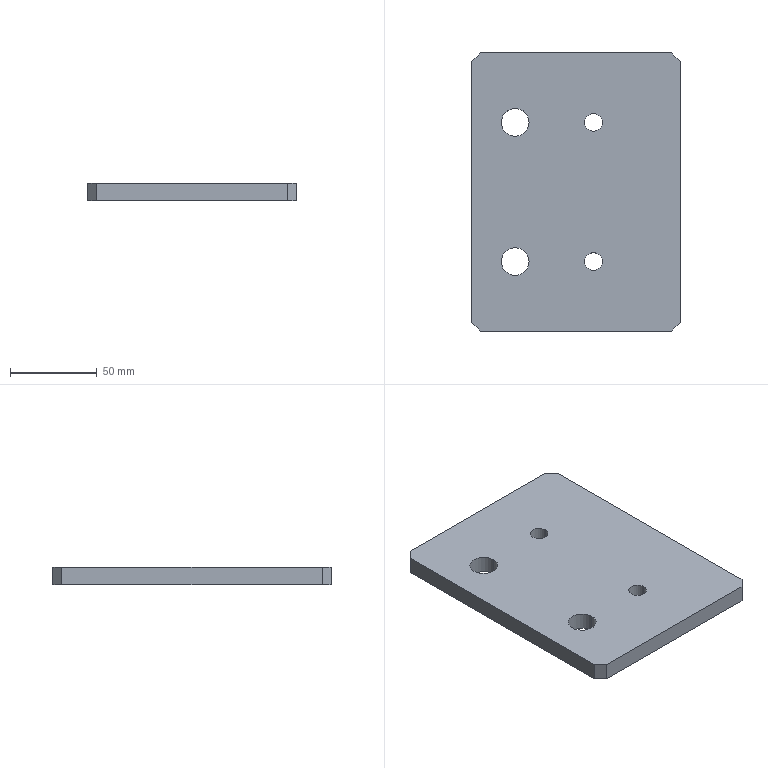Part | STEP file | 中转釜楼梯底Plate 1 | 1 solid | 18 faces | box 120 x 160 x 10 mm | volume 185845 mm3 | plane 10 | cylinder 8 | commonest cylinder face diameters 10.2 x4 16 x4
STEP:
#1=CARTESIAN_POINT('',(0.,0.,0.));
#2=DIRECTION('',(0.,0.,1.));
#3=DIRECTION('',(1.,0.,0.));
#4=AXIS2_PLACEMENT_3D('',#1,#2,#3);
#5=CARTESIAN_POINT('',(15.1,120.,0.));
#6=VERTEX_POINT('',#5);
#7=CARTESIAN_POINT('',(15.1,120.,10.));
#8=VERTEX_POINT('',#7);
#9=CARTESIAN_POINT('',(15.1,120.,10.));
#10=DIRECTION('',(0.,0.,1.));
#11=VECTOR('',#10,1.);
#12=LINE('',#9,#11);
#13=CARTESIAN_POINT('',(10.,120.,10.));
#14=DIRECTION('',(0.,0.,1.));
#15=DIRECTION('',(1.,0.,0.));
#16=AXIS2_PLACEMENT_3D('',#13,#14,#15);
#17=CYLINDRICAL_SURFACE('',#16,5.1);
#18=CARTESIAN_POINT('',(6.283,0.));
#19=DIRECTION('',(0.,1.));
#20=VECTOR('',#19,1.);
#21=LINE('',#18,#20);
#22=(GEOMETRIC_REPRESENTATION_CONTEXT(2)PARAMETRIC_REPRESENTATION_CONTEXT()REPRESENTATION_CONTEXT('',''));
#23=DEFINITIONAL_REPRESENTATION('',(#21),#22);
#24=PCURVE('',#17,#23);
#25=CARTESIAN_POINT('',(10.,120.,10.));
#26=DIRECTION('',(0.,0.,1.));
#27=DIRECTION('',(1.,0.,0.));
#28=AXIS2_PLACEMENT_3D('',#25,#26,#27);
#29=CYLINDRICAL_SURFACE('',#28,5.1);
#30=CARTESIAN_POINT('',(0.,0.));
#31=DIRECTION('',(0.,1.));
#32=VECTOR('',#31,1.);
#33=LINE('',#30,#32);
#34=(GEOMETRIC_REPRESENTATION_CONTEXT(2)PARAMETRIC_REPRESENTATION_CONTEXT()REPRESENTATION_CONTEXT('',''));
#35=DEFINITIONAL_REPRESENTATION('',(#33),#34);
#36=PCURVE('',#29,#35);
#37=SURFACE_CURVE('',#12,(#24,#36),.PCURVE_S1.);
#38=EDGE_CURVE('',#6,#8,#37,.T.);
#39=ORIENTED_EDGE('',*,*,#38,.T.);
#40=CARTESIAN_POINT('',(4.9,120.,10.));
#41=VERTEX_POINT('',#40);
#42=CARTESIAN_POINT('',(10.,120.,10.));
#43=DIRECTION('',(0.,0.,1.));
#44=DIRECTION('',(1.,0.,0.));
#45=AXIS2_PLACEMENT_3D('',#42,#43,#44);
#46=CIRCLE('',#45,5.1);
#47=CARTESIAN_POINT('',(0.,0.));
#48=DIRECTION('',(1.,0.));
#49=VECTOR('',#48,1.);
#50=LINE('',#47,#49);
#51=(GEOMETRIC_REPRESENTATION_CONTEXT(2)PARAMETRIC_REPRESENTATION_CONTEXT()REPRESENTATION_CONTEXT('',''));
#52=DEFINITIONAL_REPRESENTATION('',(#50),#51);
#53=PCURVE('',#17,#52);
#54=CARTESIAN_POINT('',(0.,0.,10.));
#55=DIRECTION('',(0.,0.,1.));
#56=DIRECTION('',(1.,0.,0.));
#57=AXIS2_PLACEMENT_3D('',#54,#55,#56);
#58=PLANE('',#57);
#59=CARTESIAN_POINT('',(10.,120.));
#60=DIRECTION('',(1.,0.));
#61=AXIS2_PLACEMENT_2D('',#59,#60);
#62=CIRCLE('',#61,5.1);
#63=(GEOMETRIC_REPRESENTATION_CONTEXT(2)PARAMETRIC_REPRESENTATION_CONTEXT()REPRESENTATION_CONTEXT('',''));
#64=DEFINITIONAL_REPRESENTATION('',(#62),#63);
#65=PCURVE('',#58,#64);
#66=SURFACE_CURVE('',#46,(#53,#65),.PCURVE_S1.);
#67=EDGE_CURVE('',#41,#8,#66,.T.);
#68=ORIENTED_EDGE('',*,*,#67,.F.);
#69=CARTESIAN_POINT('',(4.9,120.,0.));
#70=VERTEX_POINT('',#69);
#71=CARTESIAN_POINT('',(4.9,120.,10.));
#72=DIRECTION('',(0.,0.,1.));
#73=VECTOR('',#72,1.);
#74=LINE('',#71,#73);
#75=CARTESIAN_POINT('',(3.142,0.));
#76=DIRECTION('',(0.,1.));
#77=VECTOR('',#76,1.);
#78=LINE('',#75,#77);
#79=(GEOMETRIC_REPRESENTATION_CONTEXT(2)PARAMETRIC_REPRESENTATION_CONTEXT()REPRESENTATION_CONTEXT('',''));
#80=DEFINITIONAL_REPRESENTATION('',(#78),#79);
#81=PCURVE('',#17,#80);
#82=CARTESIAN_POINT('',(3.142,0.));
#83=DIRECTION('',(0.,1.));
#84=VECTOR('',#83,1.);
#85=LINE('',#82,#84);
#86=(GEOMETRIC_REPRESENTATION_CONTEXT(2)PARAMETRIC_REPRESENTATION_CONTEXT()REPRESENTATION_CONTEXT('',''));
#87=DEFINITIONAL_REPRESENTATION('',(#85),#86);
#88=PCURVE('',#29,#87);
#89=SURFACE_CURVE('',#74,(#81,#88),.PCURVE_S1.);
#90=EDGE_CURVE('',#70,#41,#89,.T.);
#91=ORIENTED_EDGE('',*,*,#90,.F.);
#92=CARTESIAN_POINT('',(10.,120.,0.));
#93=DIRECTION('',(0.,0.,1.));
#94=DIRECTION('',(1.,0.,0.));
#95=AXIS2_PLACEMENT_3D('',#92,#93,#94);
#96=CIRCLE('',#95,5.1);
#97=CARTESIAN_POINT('',(0.,-10.));
#98=DIRECTION('',(1.,0.));
#99=VECTOR('',#98,1.);
#100=LINE('',#97,#99);
#101=(GEOMETRIC_REPRESENTATION_CONTEXT(2)PARAMETRIC_REPRESENTATION_CONTEXT()REPRESENTATION_CONTEXT('',''));
#102=DEFINITIONAL_REPRESENTATION('',(#100),#101);
#103=PCURVE('',#17,#102);
#104=CARTESIAN_POINT('',(0.,0.,0.));
#105=DIRECTION('',(0.,0.,1.));
#106=DIRECTION('',(1.,0.,0.));
#107=AXIS2_PLACEMENT_3D('',#104,#105,#106);
#108=PLANE('',#107);
#109=CARTESIAN_POINT('',(10.,120.));
#110=DIRECTION('',(1.,0.));
#111=AXIS2_PLACEMENT_2D('',#109,#110);
#112=CIRCLE('',#111,5.1);
#113=(GEOMETRIC_REPRESENTATION_CONTEXT(2)PARAMETRIC_REPRESENTATION_CONTEXT()REPRESENTATION_CONTEXT('',''));
#114=DEFINITIONAL_REPRESENTATION('',(#112),#113);
#115=PCURVE('',#108,#114);
#116=SURFACE_CURVE('',#96,(#103,#115),.PCURVE_S1.);
#117=EDGE_CURVE('',#70,#6,#116,.T.);
#118=ORIENTED_EDGE('',*,*,#117,.T.);
#119=EDGE_LOOP('',(#39,#68,#91,#118));
#120=FACE_BOUND('',#119,.F.);
#121=ADVANCED_FACE('',(#120),#17,.F.);
#122=CARTESIAN_POINT('',(15.1,40.,0.));
#123=VERTEX_POINT('',#122);
#124=CARTESIAN_POINT('',(15.1,40.,10.));
#125=VERTEX_POINT('',#124);
#126=CARTESIAN_POINT('',(15.1,40.,10.));
#127=DIRECTION('',(0.,0.,1.));
#128=VECTOR('',#127,1.);
#129=LINE('',#126,#128);
#130=CARTESIAN_POINT('',(10.,40.,10.));
#131=DIRECTION('',(0.,0.,1.));
#132=DIRECTION('',(1.,0.,0.));
#133=AXIS2_PLACEMENT_3D('',#130,#131,#132);
#134=CYLINDRICAL_SURFACE('',#133,5.1);
#135=CARTESIAN_POINT('',(6.283,0.));
#136=DIRECTION('',(0.,1.));
#137=VECTOR('',#136,1.);
#138=LINE('',#135,#137);
#139=(GEOMETRIC_REPRESENTATION_CONTEXT(2)PARAMETRIC_REPRESENTATION_CONTEXT()REPRESENTATION_CONTEXT('',''));
#140=DEFINITIONAL_REPRESENTATION('',(#138),#139);
#141=PCURVE('',#134,#140);
#142=CARTESIAN_POINT('',(10.,40.,10.));
#143=DIRECTION('',(0.,0.,1.));
#144=DIRECTION('',(1.,0.,0.));
#145=AXIS2_PLACEMENT_3D('',#142,#143,#144);
#146=CYLINDRICAL_SURFACE('',#145,5.1);
#147=CARTESIAN_POINT('',(0.,0.));
#148=DIRECTION('',(0.,1.));
#149=VECTOR('',#148,1.);
#150=LINE('',#147,#149);
#151=(GEOMETRIC_REPRESENTATION_CONTEXT(2)PARAMETRIC_REPRESENTATION_CONTEXT()REPRESENTATION_CONTEXT('',''));
#152=DEFINITIONAL_REPRESENTATION('',(#150),#151);
#153=PCURVE('',#146,#152);
#154=SURFACE_CURVE('',#129,(#141,#153),.PCURVE_S1.);
#155=EDGE_CURVE('',#123,#125,#154,.T.);
#156=ORIENTED_EDGE('',*,*,#155,.T.);
#157=CARTESIAN_POINT('',(4.9,40.,10.));
#158=VERTEX_POINT('',#157);
#159=CARTESIAN_POINT('',(10.,40.,10.));
#160=DIRECTION('',(0.,0.,1.));
#161=DIRECTION('',(1.,0.,0.));
#162=AXIS2_PLACEMENT_3D('',#159,#160,#161);
#163=CIRCLE('',#162,5.1);
#164=CARTESIAN_POINT('',(0.,0.));
#165=DIRECTION('',(1.,0.));
#166=VECTOR('',#165,1.);
#167=LINE('',#164,#166);
#168=(GEOMETRIC_REPRESENTATION_CONTEXT(2)PARAMETRIC_REPRESENTATION_CONTEXT()REPRESENTATION_CONTEXT('',''));
#169=DEFINITIONAL_REPRESENTATION('',(#167),#168);
#170=PCURVE('',#134,#169);
#171=CARTESIAN_POINT('',(10.,40.));
#172=DIRECTION('',(1.,0.));
#173=AXIS2_PLACEMENT_2D('',#171,#172);
#174=CIRCLE('',#173,5.1);
#175=(GEOMETRIC_REPRESENTATION_CONTEXT(2)PARAMETRIC_REPRESENTATION_CONTEXT()REPRESENTATION_CONTEXT('',''));
#176=DEFINITIONAL_REPRESENTATION('',(#174),#175);
#177=PCURVE('',#58,#176);
#178=SURFACE_CURVE('',#163,(#170,#177),.PCURVE_S1.);
#179=EDGE_CURVE('',#158,#125,#178,.T.);
#180=ORIENTED_EDGE('',*,*,#179,.F.);
#181=CARTESIAN_POINT('',(4.9,40.,0.));
#182=VERTEX_POINT('',#181);
#183=CARTESIAN_POINT('',(4.9,40.,10.));
#184=DIRECTION('',(0.,0.,1.));
#185=VECTOR('',#184,1.);
#186=LINE('',#183,#185);
#187=CARTESIAN_POINT('',(3.142,0.));
#188=DIRECTION('',(0.,1.));
#189=VECTOR('',#188,1.);
#190=LINE('',#187,#189);
#191=(GEOMETRIC_REPRESENTATION_CONTEXT(2)PARAMETRIC_REPRESENTATION_CONTEXT()REPRESENTATION_CONTEXT('',''));
#192=DEFINITIONAL_REPRESENTATION('',(#190),#191);
#193=PCURVE('',#134,#192);
#194=CARTESIAN_POINT('',(3.142,0.));
#195=DIRECTION('',(0.,1.));
#196=VECTOR('',#195,1.);
#197=LINE('',#194,#196);
#198=(GEOMETRIC_REPRESENTATION_CONTEXT(2)PARAMETRIC_REPRESENTATION_CONTEXT()REPRESENTATION_CONTEXT('',''));
#199=DEFINITIONAL_REPRESENTATION('',(#197),#198);
#200=PCURVE('',#146,#199);
#201=SURFACE_CURVE('',#186,(#193,#200),.PCURVE_S1.);
#202=EDGE_CURVE('',#182,#158,#201,.T.);
#203=ORIENTED_EDGE('',*,*,#202,.F.);
#204=CARTESIAN_POINT('',(10.,40.,0.));
#205=DIRECTION('',(0.,0.,1.));
#206=DIRECTION('',(1.,0.,0.));
#207=AXIS2_PLACEMENT_3D('',#204,#205,#206);
#208=CIRCLE('',#207,5.1);
#209=CARTESIAN_POINT('',(0.,-10.));
#210=DIRECTION('',(1.,0.));
#211=VECTOR('',#210,1.);
#212=LINE('',#209,#211);
#213=(GEOMETRIC_REPRESENTATION_CONTEXT(2)PARAMETRIC_REPRESENTATION_CONTEXT()REPRESENTATION_CONTEXT('',''));
#214=DEFINITIONAL_REPRESENTATION('',(#212),#213);
#215=PCURVE('',#134,#214);
#216=CARTESIAN_POINT('',(10.,40.));
#217=DIRECTION('',(1.,0.));
#218=AXIS2_PLACEMENT_2D('',#216,#217);
#219=CIRCLE('',#218,5.1);
#220=(GEOMETRIC_REPRESENTATION_CONTEXT(2)PARAMETRIC_REPRESENTATION_CONTEXT()REPRESENTATION_CONTEXT('',''));
#221=DEFINITIONAL_REPRESENTATION('',(#219),#220);
#222=PCURVE('',#108,#221);
#223=SURFACE_CURVE('',#208,(#215,#222),.PCURVE_S1.);
#224=EDGE_CURVE('',#182,#123,#223,.T.);
#225=ORIENTED_EDGE('',*,*,#224,.T.);
#226=EDGE_LOOP('',(#156,#180,#203,#225));
#227=FACE_BOUND('',#226,.F.);
#228=ADVANCED_FACE('',(#227),#134,.F.);
#229=CARTESIAN_POINT('',(-27.,40.,0.));
#230=VERTEX_POINT('',#229);
#231=CARTESIAN_POINT('',(-27.,40.,10.));
#232=VERTEX_POINT('',#231);
#233=CARTESIAN_POINT('',(-27.,40.,10.));
#234=DIRECTION('',(0.,0.,1.));
#235=VECTOR('',#234,1.);
#236=LINE('',#233,#235);
#237=CARTESIAN_POINT('',(-35.,40.,10.));
#238=DIRECTION('',(0.,0.,1.));
#239=DIRECTION('',(1.,0.,0.));
#240=AXIS2_PLACEMENT_3D('',#237,#238,#239);
#241=CYLINDRICAL_SURFACE('',#240,8.);
#242=CARTESIAN_POINT('',(6.283,0.));
#243=DIRECTION('',(0.,1.));
#244=VECTOR('',#243,1.);
#245=LINE('',#242,#244);
#246=(GEOMETRIC_REPRESENTATION_CONTEXT(2)PARAMETRIC_REPRESENTATION_CONTEXT()REPRESENTATION_CONTEXT('',''));
#247=DEFINITIONAL_REPRESENTATION('',(#245),#246);
#248=PCURVE('',#241,#247);
#249=CARTESIAN_POINT('',(-35.,40.,10.));
#250=DIRECTION('',(0.,0.,1.));
#251=DIRECTION('',(1.,0.,0.));
#252=AXIS2_PLACEMENT_3D('',#249,#250,#251);
#253=CYLINDRICAL_SURFACE('',#252,8.);
#254=CARTESIAN_POINT('',(0.,0.));
#255=DIRECTION('',(0.,1.));
#256=VECTOR('',#255,1.);
#257=LINE('',#254,#256);
#258=(GEOMETRIC_REPRESENTATION_CONTEXT(2)PARAMETRIC_REPRESENTATION_CONTEXT()REPRESENTATION_CONTEXT('',''));
#259=DEFINITIONAL_REPRESENTATION('',(#257),#258);
#260=PCURVE('',#253,#259);
#261=SURFACE_CURVE('',#236,(#248,#260),.PCURVE_S1.);
#262=EDGE_CURVE('',#230,#232,#261,.T.);
#263=ORIENTED_EDGE('',*,*,#262,.T.);
#264=CARTESIAN_POINT('',(-43.,40.,10.));
#265=VERTEX_POINT('',#264);
#266=CARTESIAN_POINT('',(-35.,40.,10.));
#267=DIRECTION('',(0.,0.,1.));
#268=DIRECTION('',(1.,0.,0.));
#269=AXIS2_PLACEMENT_3D('',#266,#267,#268);
#270=CIRCLE('',#269,8.);
#271=CARTESIAN_POINT('',(0.,0.));
#272=DIRECTION('',(1.,0.));
#273=VECTOR('',#272,1.);
#274=LINE('',#271,#273);
#275=(GEOMETRIC_REPRESENTATION_CONTEXT(2)PARAMETRIC_REPRESENTATION_CONTEXT()REPRESENTATION_CONTEXT('',''));
#276=DEFINITIONAL_REPRESENTATION('',(#274),#275);
#277=PCURVE('',#241,#276);
#278=CARTESIAN_POINT('',(-35.,40.));
#279=DIRECTION('',(1.,0.));
#280=AXIS2_PLACEMENT_2D('',#278,#279);
#281=CIRCLE('',#280,8.);
#282=(GEOMETRIC_REPRESENTATION_CONTEXT(2)PARAMETRIC_REPRESENTATION_CONTEXT()REPRESENTATION_CONTEXT('',''));
#283=DEFINITIONAL_REPRESENTATION('',(#281),#282);
#284=PCURVE('',#58,#283);
#285=SURFACE_CURVE('',#270,(#277,#284),.PCURVE_S1.);
#286=EDGE_CURVE('',#265,#232,#285,.T.);
#287=ORIENTED_EDGE('',*,*,#286,.F.);
#288=CARTESIAN_POINT('',(-43.,40.,0.));
#289=VERTEX_POINT('',#288);
#290=CARTESIAN_POINT('',(-43.,40.,10.));
#291=DIRECTION('',(0.,0.,1.));
#292=VECTOR('',#291,1.);
#293=LINE('',#290,#292);
#294=CARTESIAN_POINT('',(3.142,0.));
#295=DIRECTION('',(0.,1.));
#296=VECTOR('',#295,1.);
#297=LINE('',#294,#296);
#298=(GEOMETRIC_REPRESENTATION_CONTEXT(2)PARAMETRIC_REPRESENTATION_CONTEXT()REPRESENTATION_CONTEXT('',''));
#299=DEFINITIONAL_REPRESENTATION('',(#297),#298);
#300=PCURVE('',#241,#299);
#301=CARTESIAN_POINT('',(3.142,0.));
#302=DIRECTION('',(0.,1.));
#303=VECTOR('',#302,1.);
#304=LINE('',#301,#303);
#305=(GEOMETRIC_REPRESENTATION_CONTEXT(2)PARAMETRIC_REPRESENTATION_CONTEXT()REPRESENTATION_CONTEXT('',''));
#306=DEFINITIONAL_REPRESENTATION('',(#304),#305);
#307=PCURVE('',#253,#306);
#308=SURFACE_CURVE('',#293,(#300,#307),.PCURVE_S1.);
#309=EDGE_CURVE('',#289,#265,#308,.T.);
#310=ORIENTED_EDGE('',*,*,#309,.F.);
#311=CARTESIAN_POINT('',(-35.,40.,0.));
#312=DIRECTION('',(0.,0.,1.));
#313=DIRECTION('',(1.,0.,0.));
#314=AXIS2_PLACEMENT_3D('',#311,#312,#313);
#315=CIRCLE('',#314,8.);
#316=CARTESIAN_POINT('',(0.,-10.));
#317=DIRECTION('',(1.,0.));
#318=VECTOR('',#317,1.);
#319=LINE('',#316,#318);
#320=(GEOMETRIC_REPRESENTATION_CONTEXT(2)PARAMETRIC_REPRESENTATION_CONTEXT()REPRESENTATION_CONTEXT('',''));
#321=DEFINITIONAL_REPRESENTATION('',(#319),#320);
#322=PCURVE('',#241,#321);
#323=CARTESIAN_POINT('',(-35.,40.));
#324=DIRECTION('',(1.,0.));
#325=AXIS2_PLACEMENT_2D('',#323,#324);
#326=CIRCLE('',#325,8.);
#327=(GEOMETRIC_REPRESENTATION_CONTEXT(2)PARAMETRIC_REPRESENTATION_CONTEXT()REPRESENTATION_CONTEXT('',''));
#328=DEFINITIONAL_REPRESENTATION('',(#326),#327);
#329=PCURVE('',#108,#328);
#330=SURFACE_CURVE('',#315,(#322,#329),.PCURVE_S1.);
#331=EDGE_CURVE('',#289,#230,#330,.T.);
#332=ORIENTED_EDGE('',*,*,#331,.T.);
#333=EDGE_LOOP('',(#263,#287,#310,#332));
#334=FACE_BOUND('',#333,.F.);
#335=ADVANCED_FACE('',(#334),#241,.F.);
#336=CARTESIAN_POINT('',(-27.,120.,0.));
#337=VERTEX_POINT('',#336);
#338=CARTESIAN_POINT('',(-27.,120.,10.));
#339=VERTEX_POINT('',#338);
#340=CARTESIAN_POINT('',(-27.,120.,10.));
#341=DIRECTION('',(0.,0.,1.));
#342=VECTOR('',#341,1.);
#343=LINE('',#340,#342);
#344=CARTESIAN_POINT('',(-35.,120.,10.));
#345=DIRECTION('',(0.,0.,1.));
#346=DIRECTION('',(1.,0.,0.));
#347=AXIS2_PLACEMENT_3D('',#344,#345,#346);
#348=CYLINDRICAL_SURFACE('',#347,8.);
#349=CARTESIAN_POINT('',(6.283,0.));
#350=DIRECTION('',(0.,1.));
#351=VECTOR('',#350,1.);
#352=LINE('',#349,#351);
#353=(GEOMETRIC_REPRESENTATION_CONTEXT(2)PARAMETRIC_REPRESENTATION_CONTEXT()REPRESENTATION_CONTEXT('',''));
#354=DEFINITIONAL_REPRESENTATION('',(#352),#353);
#355=PCURVE('',#348,#354);
#356=CARTESIAN_POINT('',(-35.,120.,10.));
#357=DIRECTION('',(0.,0.,1.));
#358=DIRECTION('',(1.,0.,0.));
#359=AXIS2_PLACEMENT_3D('',#356,#357,#358);
#360=CYLINDRICAL_SURFACE('',#359,8.);
#361=CARTESIAN_POINT('',(0.,0.));
#362=DIRECTION('',(0.,1.));
#363=VECTOR('',#362,1.);
#364=LINE('',#361,#363);
#365=(GEOMETRIC_REPRESENTATION_CONTEXT(2)PARAMETRIC_REPRESENTATION_CONTEXT()REPRESENTATION_CONTEXT('',''));
#366=DEFINITIONAL_REPRESENTATION('',(#364),#365);
#367=PCURVE('',#360,#366);
#368=SURFACE_CURVE('',#343,(#355,#367),.PCURVE_S1.);
#369=EDGE_CURVE('',#337,#339,#368,.T.);
#370=ORIENTED_EDGE('',*,*,#369,.T.);
#371=CARTESIAN_POINT('',(-43.,120.,10.));
#372=VERTEX_POINT('',#371);
#373=CARTESIAN_POINT('',(-35.,120.,10.));
#374=DIRECTION('',(0.,0.,1.));
#375=DIRECTION('',(1.,0.,0.));
#376=AXIS2_PLACEMENT_3D('',#373,#374,#375);
#377=CIRCLE('',#376,8.);
#378=CARTESIAN_POINT('',(0.,0.));
#379=DIRECTION('',(1.,0.));
#380=VECTOR('',#379,1.);
#381=LINE('',#378,#380);
#382=(GEOMETRIC_REPRESENTATION_CONTEXT(2)PARAMETRIC_REPRESENTATION_CONTEXT()REPRESENTATION_CONTEXT('',''));
#383=DEFINITIONAL_REPRESENTATION('',(#381),#382);
#384=PCURVE('',#348,#383);
#385=CARTESIAN_POINT('',(-35.,120.));
#386=DIRECTION('',(1.,0.));
#387=AXIS2_PLACEMENT_2D('',#385,#386);
#388=CIRCLE('',#387,8.);
#389=(GEOMETRIC_REPRESENTATION_CONTEXT(2)PARAMETRIC_REPRESENTATION_CONTEXT()REPRESENTATION_CONTEXT('',''));
#390=DEFINITIONAL_REPRESENTATION('',(#388),#389);
#391=PCURVE('',#58,#390);
#392=SURFACE_CURVE('',#377,(#384,#391),.PCURVE_S1.);
#393=EDGE_CURVE('',#372,#339,#392,.T.);
#394=ORIENTED_EDGE('',*,*,#393,.F.);
#395=CARTESIAN_POINT('',(-43.,120.,0.));
#396=VERTEX_POINT('',#395);
#397=CARTESIAN_POINT('',(-43.,120.,10.));
#398=DIRECTION('',(0.,0.,1.));
#399=VECTOR('',#398,1.);
#400=LINE('',#397,#399);
#401=CARTESIAN_POINT('',(3.142,0.));
#402=DIRECTION('',(0.,1.));
#403=VECTOR('',#402,1.);
#404=LINE('',#401,#403);
#405=(GEOMETRIC_REPRESENTATION_CONTEXT(2)PARAMETRIC_REPRESENTATION_CONTEXT()REPRESENTATION_CONTEXT('',''));
#406=DEFINITIONAL_REPRESENTATION('',(#404),#405);
#407=PCURVE('',#348,#406);
#408=CARTESIAN_POINT('',(3.142,0.));
#409=DIRECTION('',(0.,1.));
#410=VECTOR('',#409,1.);
#411=LINE('',#408,#410);
#412=(GEOMETRIC_REPRESENTATION_CONTEXT(2)PARAMETRIC_REPRESENTATION_CONTEXT()REPRESENTATION_CONTEXT('',''));
#413=DEFINITIONAL_REPRESENTATION('',(#411),#412);
#414=PCURVE('',#360,#413);
#415=SURFACE_CURVE('',#400,(#407,#414),.PCURVE_S1.);
#416=EDGE_CURVE('',#396,#372,#415,.T.);
#417=ORIENTED_EDGE('',*,*,#416,.F.);
#418=CARTESIAN_POINT('',(-35.,120.,0.));
#419=DIRECTION('',(0.,0.,1.));
#420=DIRECTION('',(1.,0.,0.));
#421=AXIS2_PLACEMENT_3D('',#418,#419,#420);
#422=CIRCLE('',#421,8.);
#423=CARTESIAN_POINT('',(0.,-10.));
#424=DIRECTION('',(1.,0.));
#425=VECTOR('',#424,1.);
#426=LINE('',#423,#425);
#427=(GEOMETRIC_REPRESENTATION_CONTEXT(2)PARAMETRIC_REPRESENTATION_CONTEXT()REPRESENTATION_CONTEXT('',''));
#428=DEFINITIONAL_REPRESENTATION('',(#426),#427);
#429=PCURVE('',#348,#428);
#430=CARTESIAN_POINT('',(-35.,120.));
#431=DIRECTION('',(1.,0.));
#432=AXIS2_PLACEMENT_2D('',#430,#431);
#433=CIRCLE('',#432,8.);
#434=(GEOMETRIC_REPRESENTATION_CONTEXT(2)PARAMETRIC_REPRESENTATION_CONTEXT()REPRESENTATION_CONTEXT('',''));
#435=DEFINITIONAL_REPRESENTATION('',(#433),#434);
#436=PCURVE('',#108,#435);
#437=SURFACE_CURVE('',#422,(#429,#436),.PCURVE_S1.);
#438=EDGE_CURVE('',#396,#337,#437,.T.);
#439=ORIENTED_EDGE('',*,*,#438,.T.);
#440=EDGE_LOOP('',(#370,#394,#417,#439));
#441=FACE_BOUND('',#440,.F.);
#442=ADVANCED_FACE('',(#441),#348,.F.);
#443=CARTESIAN_POINT('',(-60.,155.,0.));
#444=VERTEX_POINT('',#443);
#445=CARTESIAN_POINT('',(-60.,5.,0.));
#446=VERTEX_POINT('',#445);
#447=CARTESIAN_POINT('',(-60.,160.,0.));
#448=DIRECTION('',(0.,-1.,0.));
#449=VECTOR('',#448,1.);
#450=LINE('',#447,#449);
#451=CARTESIAN_POINT('',(-60.,160.,10.));
#452=DIRECTION('',(1.,0.,0.));
#453=DIRECTION('',(0.,1.,0.));
#454=AXIS2_PLACEMENT_3D('',#451,#452,#453);
#455=PLANE('',#454);
#456=CARTESIAN_POINT('',(0.,-10.));
#457=DIRECTION('',(-1.,0.));
#458=VECTOR('',#457,1.);
#459=LINE('',#456,#458);
#460=(GEOMETRIC_REPRESENTATION_CONTEXT(2)PARAMETRIC_REPRESENTATION_CONTEXT()REPRESENTATION_CONTEXT('',''));
#461=DEFINITIONAL_REPRESENTATION('',(#459),#460);
#462=PCURVE('',#455,#461);
#463=CARTESIAN_POINT('',(-60.,160.));
#464=DIRECTION('',(0.,-1.));
#465=VECTOR('',#464,1.);
#466=LINE('',#463,#465);
#467=(GEOMETRIC_REPRESENTATION_CONTEXT(2)PARAMETRIC_REPRESENTATION_CONTEXT()REPRESENTATION_CONTEXT('',''));
#468=DEFINITIONAL_REPRESENTATION('',(#466),#467);
#469=PCURVE('',#108,#468);
#470=SURFACE_CURVE('',#450,(#462,#469),.PCURVE_S1.);
#471=EDGE_CURVE('',#444,#446,#470,.T.);
#472=ORIENTED_EDGE('',*,*,#471,.T.);
#473=CARTESIAN_POINT('',(-60.,5.,10.));
#474=VERTEX_POINT('',#473);
#475=CARTESIAN_POINT('',(-60.,5.,10.));
#476=DIRECTION('',(0.,0.,1.));
#477=VECTOR('',#476,1.);
#478=LINE('',#475,#477);
#479=CARTESIAN_POINT('',(-155.,0.));
#480=DIRECTION('',(0.,1.));
#481=VECTOR('',#480,1.);
#482=LINE('',#479,#481);
#483=(GEOMETRIC_REPRESENTATION_CONTEXT(2)PARAMETRIC_REPRESENTATION_CONTEXT()REPRESENTATION_CONTEXT('',''));
#484=DEFINITIONAL_REPRESENTATION('',(#482),#483);
#485=PCURVE('',#455,#484);
#486=CARTESIAN_POINT('',(-55.,0.,10.));
#487=DIRECTION('',(0.7071,0.7071,0.));
#488=DIRECTION('',(0.,0.,-1.));
#489=AXIS2_PLACEMENT_3D('',#486,#487,#488);
#490=PLANE('',#489);
#491=CARTESIAN_POINT('',(0.,7.071));
#492=DIRECTION('',(-1.,0.));
#493=VECTOR('',#492,1.);
#494=LINE('',#491,#493);
#495=(GEOMETRIC_REPRESENTATION_CONTEXT(2)PARAMETRIC_REPRESENTATION_CONTEXT()REPRESENTATION_CONTEXT('',''));
#496=DEFINITIONAL_REPRESENTATION('',(#494),#495);
#497=PCURVE('',#490,#496);
#498=SURFACE_CURVE('',#478,(#485,#497),.PCURVE_S1.);
#499=EDGE_CURVE('',#446,#474,#498,.T.);
#500=ORIENTED_EDGE('',*,*,#499,.T.);
#501=CARTESIAN_POINT('',(-60.,155.,10.));
#502=VERTEX_POINT('',#501);
#503=CARTESIAN_POINT('',(-60.,160.,10.));
#504=DIRECTION('',(0.,-1.,0.));
#505=VECTOR('',#504,1.);
#506=LINE('',#503,#505);
#507=CARTESIAN_POINT('',(0.,0.));
#508=DIRECTION('',(-1.,0.));
#509=VECTOR('',#508,1.);
#510=LINE('',#507,#509);
#511=(GEOMETRIC_REPRESENTATION_CONTEXT(2)PARAMETRIC_REPRESENTATION_CONTEXT()REPRESENTATION_CONTEXT('',''));
#512=DEFINITIONAL_REPRESENTATION('',(#510),#511);
#513=PCURVE('',#455,#512);
#514=CARTESIAN_POINT('',(-60.,160.));
#515=DIRECTION('',(0.,-1.));
#516=VECTOR('',#515,1.);
#517=LINE('',#514,#516);
#518=(GEOMETRIC_REPRESENTATION_CONTEXT(2)PARAMETRIC_REPRESENTATION_CONTEXT()REPRESENTATION_CONTEXT('',''));
#519=DEFINITIONAL_REPRESENTATION('',(#517),#518);
#520=PCURVE('',#58,#519);
#521=SURFACE_CURVE('',#506,(#513,#520),.PCURVE_S1.);
#522=EDGE_CURVE('',#502,#474,#521,.T.);
#523=ORIENTED_EDGE('',*,*,#522,.F.);
#524=CARTESIAN_POINT('',(-60.,155.,10.));
#525=DIRECTION('',(0.,0.,-1.));
#526=VECTOR('',#525,1.);
#527=LINE('',#524,#526);
#528=CARTESIAN_POINT('',(-5.,0.));
#529=DIRECTION('',(0.,-1.));
#530=VECTOR('',#529,1.);
#531=LINE('',#528,#530);
#532=(GEOMETRIC_REPRESENTATION_CONTEXT(2)PARAMETRIC_REPRESENTATION_CONTEXT()REPRESENTATION_CONTEXT('',''));
#533=DEFINITIONAL_REPRESENTATION('',(#531),#532);
#534=PCURVE('',#455,#533);
#535=CARTESIAN_POINT('',(-60.,155.,10.));
#536=DIRECTION('',(0.7071,-0.7071,0.));
#537=DIRECTION('',(0.,0.,-1.));
#538=AXIS2_PLACEMENT_3D('',#535,#536,#537);
#539=PLANE('',#538);
#540=CARTESIAN_POINT('',(0.,0.));
#541=DIRECTION('',(1.,0.));
#542=VECTOR('',#541,1.);
#543=LINE('',#540,#542);
#544=(GEOMETRIC_REPRESENTATION_CONTEXT(2)PARAMETRIC_REPRESENTATION_CONTEXT()REPRESENTATION_CONTEXT('',''));
#545=DEFINITIONAL_REPRESENTATION('',(#543),#544);
#546=PCURVE('',#539,#545);
#547=SURFACE_CURVE('',#527,(#534,#546),.PCURVE_S1.);
#548=EDGE_CURVE('',#502,#444,#547,.T.);
#549=ORIENTED_EDGE('',*,*,#548,.T.);
#550=EDGE_LOOP('',(#472,#500,#523,#549));
#551=FACE_BOUND('',#550,.T.);
#552=ADVANCED_FACE('',(#551),#455,.F.);
#553=CARTESIAN_POINT('',(-55.,0.,10.));
#554=VERTEX_POINT('',#553);
#555=CARTESIAN_POINT('',(55.,0.,10.));
#556=VERTEX_POINT('',#555);
#557=CARTESIAN_POINT('',(-60.,0.,10.));
#558=DIRECTION('',(1.,0.,0.));
#559=VECTOR('',#558,1.);
#560=LINE('',#557,#559);
#561=CARTESIAN_POINT('',(-60.,0.,10.));
#562=DIRECTION('',(0.,1.,0.));
#563=DIRECTION('',(0.,0.,1.));
#564=AXIS2_PLACEMENT_3D('',#561,#562,#563);
#565=PLANE('',#564);
#566=CARTESIAN_POINT('',(0.,0.));
#567=DIRECTION('',(0.,1.));
#568=VECTOR('',#567,1.);
#569=LINE('',#566,#568);
#570=(GEOMETRIC_REPRESENTATION_CONTEXT(2)PARAMETRIC_REPRESENTATION_CONTEXT()REPRESENTATION_CONTEXT('',''));
#571=DEFINITIONAL_REPRESENTATION('',(#569),#570);
#572=PCURVE('',#565,#571);
#573=CARTESIAN_POINT('',(-60.,0.));
#574=DIRECTION('',(1.,0.));
#575=VECTOR('',#574,1.);
#576=LINE('',#573,#575);
#577=(GEOMETRIC_REPRESENTATION_CONTEXT(2)PARAMETRIC_REPRESENTATION_CONTEXT()REPRESENTATION_CONTEXT('',''));
#578=DEFINITIONAL_REPRESENTATION('',(#576),#577);
#579=PCURVE('',#58,#578);
#580=SURFACE_CURVE('',#560,(#572,#579),.PCURVE_S1.);
#581=EDGE_CURVE('',#554,#556,#580,.T.);
#582=ORIENTED_EDGE('',*,*,#581,.F.);
#583=CARTESIAN_POINT('',(-55.,0.,0.));
#584=VERTEX_POINT('',#583);
#585=CARTESIAN_POINT('',(-55.,0.,10.));
#586=DIRECTION('',(0.,0.,-1.));
#587=VECTOR('',#586,1.);
#588=LINE('',#585,#587);
#589=CARTESIAN_POINT('',(0.,5.));
#590=DIRECTION('',(-1.,0.));
#591=VECTOR('',#590,1.);
#592=LINE('',#589,#591);
#593=(GEOMETRIC_REPRESENTATION_CONTEXT(2)PARAMETRIC_REPRESENTATION_CONTEXT()REPRESENTATION_CONTEXT('',''));
#594=DEFINITIONAL_REPRESENTATION('',(#592),#593);
#595=PCURVE('',#565,#594);
#596=CARTESIAN_POINT('',(0.,0.));
#597=DIRECTION('',(1.,0.));
#598=VECTOR('',#597,1.);
#599=LINE('',#596,#598);
#600=(GEOMETRIC_REPRESENTATION_CONTEXT(2)PARAMETRIC_REPRESENTATION_CONTEXT()REPRESENTATION_CONTEXT('',''));
#601=DEFINITIONAL_REPRESENTATION('',(#599),#600);
#602=PCURVE('',#490,#601);
#603=SURFACE_CURVE('',#588,(#595,#602),.PCURVE_S1.);
#604=EDGE_CURVE('',#554,#584,#603,.T.);
#605=ORIENTED_EDGE('',*,*,#604,.T.);
#606=CARTESIAN_POINT('',(55.,0.,0.));
#607=VERTEX_POINT('',#606);
#608=CARTESIAN_POINT('',(-60.,0.,0.));
#609=DIRECTION('',(1.,0.,0.));
#610=VECTOR('',#609,1.);
#611=LINE('',#608,#610);
#612=CARTESIAN_POINT('',(-10.,0.));
#613=DIRECTION('',(0.,1.));
#614=VECTOR('',#613,1.);
#615=LINE('',#612,#614);
#616=(GEOMETRIC_REPRESENTATION_CONTEXT(2)PARAMETRIC_REPRESENTATION_CONTEXT()REPRESENTATION_CONTEXT('',''));
#617=DEFINITIONAL_REPRESENTATION('',(#615),#616);
#618=PCURVE('',#565,#617);
#619=CARTESIAN_POINT('',(-60.,0.));
#620=DIRECTION('',(1.,0.));
#621=VECTOR('',#620,1.);
#622=LINE('',#619,#621);
#623=(GEOMETRIC_REPRESENTATION_CONTEXT(2)PARAMETRIC_REPRESENTATION_CONTEXT()REPRESENTATION_CONTEXT('',''));
#624=DEFINITIONAL_REPRESENTATION('',(#622),#623);
#625=PCURVE('',#108,#624);
#626=SURFACE_CURVE('',#611,(#618,#625),.PCURVE_S1.);
#627=EDGE_CURVE('',#584,#607,#626,.T.);
#628=ORIENTED_EDGE('',*,*,#627,.T.);
#629=CARTESIAN_POINT('',(55.,0.,10.));
#630=DIRECTION('',(0.,0.,1.));
#631=VECTOR('',#630,1.);
#632=LINE('',#629,#631);
#633=CARTESIAN_POINT('',(0.,115.));
#634=DIRECTION('',(1.,0.));
#635=VECTOR('',#634,1.);
#636=LINE('',#633,#635);
#637=(GEOMETRIC_REPRESENTATION_CONTEXT(2)PARAMETRIC_REPRESENTATION_CONTEXT()REPRESENTATION_CONTEXT('',''));
#638=DEFINITIONAL_REPRESENTATION('',(#636),#637);
#639=PCURVE('',#565,#638);
#640=CARTESIAN_POINT('',(60.,5.,10.));
#641=DIRECTION('',(-0.7071,0.7071,0.));
#642=DIRECTION('',(0.,0.,-1.));
#643=AXIS2_PLACEMENT_3D('',#640,#641,#642);
#644=PLANE('',#643);
#645=CARTESIAN_POINT('',(0.,7.071));
#646=DIRECTION('',(-1.,0.));
#647=VECTOR('',#646,1.);
#648=LINE('',#645,#647);
#649=(GEOMETRIC_REPRESENTATION_CONTEXT(2)PARAMETRIC_REPRESENTATION_CONTEXT()REPRESENTATION_CONTEXT('',''));
#650=DEFINITIONAL_REPRESENTATION('',(#648),#649);
#651=PCURVE('',#644,#650);
#652=SURFACE_CURVE('',#632,(#639,#651),.PCURVE_S1.);
#653=EDGE_CURVE('',#607,#556,#652,.T.);
#654=ORIENTED_EDGE('',*,*,#653,.T.);
#655=EDGE_LOOP('',(#582,#605,#628,#654));
#656=FACE_BOUND('',#655,.T.);
#657=ADVANCED_FACE('',(#656),#565,.F.);
#658=CARTESIAN_POINT('',(60.,5.,10.));
#659=VERTEX_POINT('',#658);
#660=CARTESIAN_POINT('',(60.,155.,10.));
#661=VERTEX_POINT('',#660);
#662=CARTESIAN_POINT('',(60.,160.,10.));
#663=DIRECTION('',(0.,1.,0.));
#664=VECTOR('',#663,1.);
#665=LINE('',#662,#664);
#666=CARTESIAN_POINT('',(60.,160.,10.));
#667=DIRECTION('',(-1.,0.,0.));
#668=DIRECTION('',(0.,-1.,0.));
#669=AXIS2_PLACEMENT_3D('',#666,#667,#668);
#670=PLANE('',#669);
#671=CARTESIAN_POINT('',(0.,0.));
#672=DIRECTION('',(-1.,0.));
#673=VECTOR('',#672,1.);
#674=LINE('',#671,#673);
#675=(GEOMETRIC_REPRESENTATION_CONTEXT(2)PARAMETRIC_REPRESENTATION_CONTEXT()REPRESENTATION_CONTEXT('',''));
#676=DEFINITIONAL_REPRESENTATION('',(#674),#675);
#677=PCURVE('',#670,#676);
#678=CARTESIAN_POINT('',(60.,160.));
#679=DIRECTION('',(0.,1.));
#680=VECTOR('',#679,1.);
#681=LINE('',#678,#680);
#682=(GEOMETRIC_REPRESENTATION_CONTEXT(2)PARAMETRIC_REPRESENTATION_CONTEXT()REPRESENTATION_CONTEXT('',''));
#683=DEFINITIONAL_REPRESENTATION('',(#681),#682);
#684=PCURVE('',#58,#683);
#685=SURFACE_CURVE('',#665,(#677,#684),.PCURVE_S1.);
#686=EDGE_CURVE('',#659,#661,#685,.T.);
#687=ORIENTED_EDGE('',*,*,#686,.F.);
#688=CARTESIAN_POINT('',(60.,5.,0.));
#689=VERTEX_POINT('',#688);
#690=CARTESIAN_POINT('',(60.,5.,10.));
#691=DIRECTION('',(0.,0.,-1.));
#692=VECTOR('',#691,1.);
#693=LINE('',#690,#692);
#694=CARTESIAN_POINT('',(155.,0.));
#695=DIRECTION('',(0.,-1.));
#696=VECTOR('',#695,1.);
#697=LINE('',#694,#696);
#698=(GEOMETRIC_REPRESENTATION_CONTEXT(2)PARAMETRIC_REPRESENTATION_CONTEXT()REPRESENTATION_CONTEXT('',''));
#699=DEFINITIONAL_REPRESENTATION('',(#697),#698);
#700=PCURVE('',#670,#699);
#701=CARTESIAN_POINT('',(0.,0.));
#702=DIRECTION('',(1.,0.));
#703=VECTOR('',#702,1.);
#704=LINE('',#701,#703);
#705=(GEOMETRIC_REPRESENTATION_CONTEXT(2)PARAMETRIC_REPRESENTATION_CONTEXT()REPRESENTATION_CONTEXT('',''));
#706=DEFINITIONAL_REPRESENTATION('',(#704),#705);
#707=PCURVE('',#644,#706);
#708=SURFACE_CURVE('',#693,(#700,#707),.PCURVE_S1.);
#709=EDGE_CURVE('',#659,#689,#708,.T.);
#710=ORIENTED_EDGE('',*,*,#709,.T.);
#711=CARTESIAN_POINT('',(60.,155.,0.));
#712=VERTEX_POINT('',#711);
#713=CARTESIAN_POINT('',(60.,160.,0.));
#714=DIRECTION('',(0.,1.,0.));
#715=VECTOR('',#714,1.);
#716=LINE('',#713,#715);
#717=CARTESIAN_POINT('',(0.,-10.));
#718=DIRECTION('',(-1.,0.));
#719=VECTOR('',#718,1.);
#720=LINE('',#717,#719);
#721=(GEOMETRIC_REPRESENTATION_CONTEXT(2)PARAMETRIC_REPRESENTATION_CONTEXT()REPRESENTATION_CONTEXT('',''));
#722=DEFINITIONAL_REPRESENTATION('',(#720),#721);
#723=PCURVE('',#670,#722);
#724=CARTESIAN_POINT('',(60.,160.));
#725=DIRECTION('',(0.,1.));
#726=VECTOR('',#725,1.);
#727=LINE('',#724,#726);
#728=(GEOMETRIC_REPRESENTATION_CONTEXT(2)PARAMETRIC_REPRESENTATION_CONTEXT()REPRESENTATION_CONTEXT('',''));
#729=DEFINITIONAL_REPRESENTATION('',(#727),#728);
#730=PCURVE('',#108,#729);
#731=SURFACE_CURVE('',#716,(#723,#730),.PCURVE_S1.);
#732=EDGE_CURVE('',#689,#712,#731,.T.);
#733=ORIENTED_EDGE('',*,*,#732,.T.);
#734=CARTESIAN_POINT('',(60.,155.,10.));
#735=DIRECTION('',(0.,0.,1.));
#736=VECTOR('',#735,1.);
#737=LINE('',#734,#736);
#738=CARTESIAN_POINT('',(5.,0.));
#739=DIRECTION('',(0.,1.));
#740=VECTOR('',#739,1.);
#741=LINE('',#738,#740);
#742=(GEOMETRIC_REPRESENTATION_CONTEXT(2)PARAMETRIC_REPRESENTATION_CONTEXT()REPRESENTATION_CONTEXT('',''));
#743=DEFINITIONAL_REPRESENTATION('',(#741),#742);
#744=PCURVE('',#670,#743);
#745=CARTESIAN_POINT('',(55.,160.,10.));
#746=DIRECTION('',(-0.7071,-0.7071,0.));
#747=DIRECTION('',(0.,0.,-1.));
#748=AXIS2_PLACEMENT_3D('',#745,#746,#747);
#749=PLANE('',#748);
#750=CARTESIAN_POINT('',(0.,7.071));
#751=DIRECTION('',(-1.,0.));
#752=VECTOR('',#751,1.);
#753=LINE('',#750,#752);
#754=(GEOMETRIC_REPRESENTATION_CONTEXT(2)PARAMETRIC_REPRESENTATION_CONTEXT()REPRESENTATION_CONTEXT('',''));
#755=DEFINITIONAL_REPRESENTATION('',(#753),#754);
#756=PCURVE('',#749,#755);
#757=SURFACE_CURVE('',#737,(#744,#756),.PCURVE_S1.);
#758=EDGE_CURVE('',#712,#661,#757,.T.);
#759=ORIENTED_EDGE('',*,*,#758,.T.);
#760=EDGE_LOOP('',(#687,#710,#733,#759));
#761=FACE_BOUND('',#760,.T.);
#762=ADVANCED_FACE('',(#761),#670,.F.);
#763=CARTESIAN_POINT('',(55.,160.,10.));
#764=VERTEX_POINT('',#763);
#765=CARTESIAN_POINT('',(-55.,160.,10.));
#766=VERTEX_POINT('',#765);
#767=CARTESIAN_POINT('',(-60.,160.,10.));
#768=DIRECTION('',(-1.,0.,0.));
#769=VECTOR('',#768,1.);
#770=LINE('',#767,#769);
#771=CARTESIAN_POINT('',(-60.,160.,10.));
#772=DIRECTION('',(0.,-1.,0.));
#773=DIRECTION('',(0.,0.,-1.));
#774=AXIS2_PLACEMENT_3D('',#771,#772,#773);
#775=PLANE('',#774);
#776=CARTESIAN_POINT('',(0.,0.));
#777=DIRECTION('',(0.,-1.));
#778=VECTOR('',#777,1.);
#779=LINE('',#776,#778);
#780=(GEOMETRIC_REPRESENTATION_CONTEXT(2)PARAMETRIC_REPRESENTATION_CONTEXT()REPRESENTATION_CONTEXT('',''));
#781=DEFINITIONAL_REPRESENTATION('',(#779),#780);
#782=PCURVE('',#775,#781);
#783=CARTESIAN_POINT('',(-60.,160.));
#784=DIRECTION('',(-1.,0.));
#785=VECTOR('',#784,1.);
#786=LINE('',#783,#785);
#787=(GEOMETRIC_REPRESENTATION_CONTEXT(2)PARAMETRIC_REPRESENTATION_CONTEXT()REPRESENTATION_CONTEXT('',''));
#788=DEFINITIONAL_REPRESENTATION('',(#786),#787);
#789=PCURVE('',#58,#788);
#790=SURFACE_CURVE('',#770,(#782,#789),.PCURVE_S1.);
#791=EDGE_CURVE('',#764,#766,#790,.T.);
#792=ORIENTED_EDGE('',*,*,#791,.F.);
#793=CARTESIAN_POINT('',(55.,160.,0.));
#794=VERTEX_POINT('',#793);
#795=CARTESIAN_POINT('',(55.,160.,10.));
#796=DIRECTION('',(0.,0.,-1.));
#797=VECTOR('',#796,1.);
#798=LINE('',#795,#797);
#799=CARTESIAN_POINT('',(0.,115.));
#800=DIRECTION('',(1.,0.));
#801=VECTOR('',#800,1.);
#802=LINE('',#799,#801);
#803=(GEOMETRIC_REPRESENTATION_CONTEXT(2)PARAMETRIC_REPRESENTATION_CONTEXT()REPRESENTATION_CONTEXT('',''));
#804=DEFINITIONAL_REPRESENTATION('',(#802),#803);
#805=PCURVE('',#775,#804);
#806=CARTESIAN_POINT('',(0.,0.));
#807=DIRECTION('',(1.,0.));
#808=VECTOR('',#807,1.);
#809=LINE('',#806,#808);
#810=(GEOMETRIC_REPRESENTATION_CONTEXT(2)PARAMETRIC_REPRESENTATION_CONTEXT()REPRESENTATION_CONTEXT('',''));
#811=DEFINITIONAL_REPRESENTATION('',(#809),#810);
#812=PCURVE('',#749,#811);
#813=SURFACE_CURVE('',#798,(#805,#812),.PCURVE_S1.);
#814=EDGE_CURVE('',#764,#794,#813,.T.);
#815=ORIENTED_EDGE('',*,*,#814,.T.);
#816=CARTESIAN_POINT('',(-55.,160.,0.));
#817=VERTEX_POINT('',#816);
#818=CARTESIAN_POINT('',(-60.,160.,0.));
#819=DIRECTION('',(-1.,0.,0.));
#820=VECTOR('',#819,1.);
#821=LINE('',#818,#820);
#822=CARTESIAN_POINT('',(10.,0.));
#823=DIRECTION('',(0.,-1.));
#824=VECTOR('',#823,1.);
#825=LINE('',#822,#824);
#826=(GEOMETRIC_REPRESENTATION_CONTEXT(2)PARAMETRIC_REPRESENTATION_CONTEXT()REPRESENTATION_CONTEXT('',''));
#827=DEFINITIONAL_REPRESENTATION('',(#825),#826);
#828=PCURVE('',#775,#827);
#829=CARTESIAN_POINT('',(-60.,160.));
#830=DIRECTION('',(-1.,0.));
#831=VECTOR('',#830,1.);
#832=LINE('',#829,#831);
#833=(GEOMETRIC_REPRESENTATION_CONTEXT(2)PARAMETRIC_REPRESENTATION_CONTEXT()REPRESENTATION_CONTEXT('',''));
#834=DEFINITIONAL_REPRESENTATION('',(#832),#833);
#835=PCURVE('',#108,#834);
#836=SURFACE_CURVE('',#821,(#828,#835),.PCURVE_S1.);
#837=EDGE_CURVE('',#794,#817,#836,.T.);
#838=ORIENTED_EDGE('',*,*,#837,.T.);
#839=CARTESIAN_POINT('',(-55.,160.,10.));
#840=DIRECTION('',(0.,0.,1.));
#841=VECTOR('',#840,1.);
#842=LINE('',#839,#841);
#843=CARTESIAN_POINT('',(0.,5.));
#844=DIRECTION('',(-1.,0.));
#845=VECTOR('',#844,1.);
#846=LINE('',#843,#845);
#847=(GEOMETRIC_REPRESENTATION_CONTEXT(2)PARAMETRIC_REPRESENTATION_CONTEXT()REPRESENTATION_CONTEXT('',''));
#848=DEFINITIONAL_REPRESENTATION('',(#846),#847);
#849=PCURVE('',#775,#848);
#850=CARTESIAN_POINT('',(0.,7.071));
#851=DIRECTION('',(-1.,0.));
#852=VECTOR('',#851,1.);
#853=LINE('',#850,#852);
#854=(GEOMETRIC_REPRESENTATION_CONTEXT(2)PARAMETRIC_REPRESENTATION_CONTEXT()REPRESENTATION_CONTEXT('',''));
#855=DEFINITIONAL_REPRESENTATION('',(#853),#854);
#856=PCURVE('',#539,#855);
#857=SURFACE_CURVE('',#842,(#849,#856),.PCURVE_S1.);
#858=EDGE_CURVE('',#817,#766,#857,.T.);
#859=ORIENTED_EDGE('',*,*,#858,.T.);
#860=EDGE_LOOP('',(#792,#815,#838,#859));
#861=FACE_BOUND('',#860,.T.);
#862=ADVANCED_FACE('',(#861),#775,.F.);
#863=CARTESIAN_POINT('',(10.,120.,10.));
#864=DIRECTION('',(0.,0.,1.));
#865=DIRECTION('',(1.,0.,0.));
#866=AXIS2_PLACEMENT_3D('',#863,#864,#865);
#867=CIRCLE('',#866,5.1);
#868=CARTESIAN_POINT('',(10.,120.));
#869=DIRECTION('',(1.,0.));
#870=AXIS2_PLACEMENT_2D('',#868,#869);
#871=CIRCLE('',#870,5.1);
#872=(GEOMETRIC_REPRESENTATION_CONTEXT(2)PARAMETRIC_REPRESENTATION_CONTEXT()REPRESENTATION_CONTEXT('',''));
#873=DEFINITIONAL_REPRESENTATION('',(#871),#872);
#874=PCURVE('',#58,#873);
#875=CARTESIAN_POINT('',(0.,0.));
#876=DIRECTION('',(1.,0.));
#877=VECTOR('',#876,1.);
#878=LINE('',#875,#877);
#879=(GEOMETRIC_REPRESENTATION_CONTEXT(2)PARAMETRIC_REPRESENTATION_CONTEXT()REPRESENTATION_CONTEXT('',''));
#880=DEFINITIONAL_REPRESENTATION('',(#878),#879);
#881=PCURVE('',#29,#880);
#882=SURFACE_CURVE('',#867,(#874,#881),.PCURVE_S1.);
#883=EDGE_CURVE('',#8,#41,#882,.T.);
#884=ORIENTED_EDGE('',*,*,#883,.F.);
#885=ORIENTED_EDGE('',*,*,#67,.F.);
#886=EDGE_LOOP('',(#884,#885));
#887=FACE_BOUND('',#886,.T.);
#888=CARTESIAN_POINT('',(10.,40.,10.));
#889=DIRECTION('',(0.,0.,1.));
#890=DIRECTION('',(1.,0.,0.));
#891=AXIS2_PLACEMENT_3D('',#888,#889,#890);
#892=CIRCLE('',#891,5.1);
#893=CARTESIAN_POINT('',(10.,40.));
#894=DIRECTION('',(1.,0.));
#895=AXIS2_PLACEMENT_2D('',#893,#894);
#896=CIRCLE('',#895,5.1);
#897=(GEOMETRIC_REPRESENTATION_CONTEXT(2)PARAMETRIC_REPRESENTATION_CONTEXT()REPRESENTATION_CONTEXT('',''));
#898=DEFINITIONAL_REPRESENTATION('',(#896),#897);
#899=PCURVE('',#58,#898);
#900=CARTESIAN_POINT('',(0.,0.));
#901=DIRECTION('',(1.,0.));
#902=VECTOR('',#901,1.);
#903=LINE('',#900,#902);
#904=(GEOMETRIC_REPRESENTATION_CONTEXT(2)PARAMETRIC_REPRESENTATION_CONTEXT()REPRESENTATION_CONTEXT('',''));
#905=DEFINITIONAL_REPRESENTATION('',(#903),#904);
#906=PCURVE('',#146,#905);
#907=SURFACE_CURVE('',#892,(#899,#906),.PCURVE_S1.);
#908=EDGE_CURVE('',#125,#158,#907,.T.);
#909=ORIENTED_EDGE('',*,*,#908,.F.);
#910=ORIENTED_EDGE('',*,*,#179,.F.);
#911=EDGE_LOOP('',(#909,#910));
#912=FACE_BOUND('',#911,.T.);
#913=CARTESIAN_POINT('',(-35.,40.,10.));
#914=DIRECTION('',(0.,0.,1.));
#915=DIRECTION('',(1.,0.,0.));
#916=AXIS2_PLACEMENT_3D('',#913,#914,#915);
#917=CIRCLE('',#916,8.);
#918=CARTESIAN_POINT('',(-35.,40.));
#919=DIRECTION('',(1.,0.));
#920=AXIS2_PLACEMENT_2D('',#918,#919);
#921=CIRCLE('',#920,8.);
#922=(GEOMETRIC_REPRESENTATION_CONTEXT(2)PARAMETRIC_REPRESENTATION_CONTEXT()REPRESENTATION_CONTEXT('',''));
#923=DEFINITIONAL_REPRESENTATION('',(#921),#922);
#924=PCURVE('',#58,#923);
#925=CARTESIAN_POINT('',(0.,0.));
#926=DIRECTION('',(1.,0.));
#927=VECTOR('',#926,1.);
#928=LINE('',#925,#927);
#929=(GEOMETRIC_REPRESENTATION_CONTEXT(2)PARAMETRIC_REPRESENTATION_CONTEXT()REPRESENTATION_CONTEXT('',''));
#930=DEFINITIONAL_REPRESENTATION('',(#928),#929);
#931=PCURVE('',#253,#930);
#932=SURFACE_CURVE('',#917,(#924,#931),.PCURVE_S1.);
#933=EDGE_CURVE('',#232,#265,#932,.T.);
#934=ORIENTED_EDGE('',*,*,#933,.F.);
#935=ORIENTED_EDGE('',*,*,#286,.F.);
#936=EDGE_LOOP('',(#934,#935));
#937=FACE_BOUND('',#936,.T.);
#938=CARTESIAN_POINT('',(-35.,120.,10.));
#939=DIRECTION('',(0.,0.,1.));
#940=DIRECTION('',(1.,0.,0.));
#941=AXIS2_PLACEMENT_3D('',#938,#939,#940);
#942=CIRCLE('',#941,8.);
#943=CARTESIAN_POINT('',(-35.,120.));
#944=DIRECTION('',(1.,0.));
#945=AXIS2_PLACEMENT_2D('',#943,#944);
#946=CIRCLE('',#945,8.);
#947=(GEOMETRIC_REPRESENTATION_CONTEXT(2)PARAMETRIC_REPRESENTATION_CONTEXT()REPRESENTATION_CONTEXT('',''));
#948=DEFINITIONAL_REPRESENTATION('',(#946),#947);
#949=PCURVE('',#58,#948);
#950=CARTESIAN_POINT('',(0.,0.));
#951=DIRECTION('',(1.,0.));
#952=VECTOR('',#951,1.);
#953=LINE('',#950,#952);
#954=(GEOMETRIC_REPRESENTATION_CONTEXT(2)PARAMETRIC_REPRESENTATION_CONTEXT()REPRESENTATION_CONTEXT('',''));
#955=DEFINITIONAL_REPRESENTATION('',(#953),#954);
#956=PCURVE('',#360,#955);
#957=SURFACE_CURVE('',#942,(#949,#956),.PCURVE_S1.);
#958=EDGE_CURVE('',#339,#372,#957,.T.);
#959=ORIENTED_EDGE('',*,*,#958,.F.);
#960=ORIENTED_EDGE('',*,*,#393,.F.);
#961=EDGE_LOOP('',(#959,#960));
#962=FACE_BOUND('',#961,.T.);
#963=ORIENTED_EDGE('',*,*,#522,.T.);
#964=CARTESIAN_POINT('',(-27.5,-27.5,10.));
#965=DIRECTION('',(0.7071,-0.7071,0.));
#966=VECTOR('',#965,1.);
#967=LINE('',#964,#966);
#968=CARTESIAN_POINT('',(-27.5,-27.5));
#969=DIRECTION('',(0.7071,-0.7071));
#970=VECTOR('',#969,1.);
#971=LINE('',#968,#970);
#972=(GEOMETRIC_REPRESENTATION_CONTEXT(2)PARAMETRIC_REPRESENTATION_CONTEXT()REPRESENTATION_CONTEXT('',''));
#973=DEFINITIONAL_REPRESENTATION('',(#971),#972);
#974=PCURVE('',#58,#973);
#975=CARTESIAN_POINT('',(0.,-38.891));
#976=DIRECTION('',(0.,-1.));
#977=VECTOR('',#976,1.);
#978=LINE('',#975,#977);
#979=(GEOMETRIC_REPRESENTATION_CONTEXT(2)PARAMETRIC_REPRESENTATION_CONTEXT()REPRESENTATION_CONTEXT('',''));
#980=DEFINITIONAL_REPRESENTATION('',(#978),#979);
#981=PCURVE('',#490,#980);
#982=SURFACE_CURVE('',#967,(#974,#981),.PCURVE_S1.);
#983=EDGE_CURVE('',#474,#554,#982,.T.);
#984=ORIENTED_EDGE('',*,*,#983,.T.);
#985=ORIENTED_EDGE('',*,*,#581,.T.);
#986=CARTESIAN_POINT('',(27.5,-27.5,10.));
#987=DIRECTION('',(0.7071,0.7071,0.));
#988=VECTOR('',#987,1.);
#989=LINE('',#986,#988);
#990=CARTESIAN_POINT('',(27.5,-27.5));
#991=DIRECTION('',(0.7071,0.7071));
#992=VECTOR('',#991,1.);
#993=LINE('',#990,#992);
#994=(GEOMETRIC_REPRESENTATION_CONTEXT(2)PARAMETRIC_REPRESENTATION_CONTEXT()REPRESENTATION_CONTEXT('',''));
#995=DEFINITIONAL_REPRESENTATION('',(#993),#994);
#996=PCURVE('',#58,#995);
#997=CARTESIAN_POINT('',(0.,45.962));
#998=DIRECTION('',(0.,-1.));
#999=VECTOR('',#998,1.);
#1000=LINE('',#997,#999);
#1001=(GEOMETRIC_REPRESENTATION_CONTEXT(2)PARAMETRIC_REPRESENTATION_CONTEXT()REPRESENTATION_CONTEXT('',''));
#1002=DEFINITIONAL_REPRESENTATION('',(#1000),#1001);
#1003=PCURVE('',#644,#1002);
#1004=SURFACE_CURVE('',#989,(#996,#1003),.PCURVE_S1.);
#1005=EDGE_CURVE('',#556,#659,#1004,.T.);
#1006=ORIENTED_EDGE('',*,*,#1005,.T.);
#1007=ORIENTED_EDGE('',*,*,#686,.T.);
#1008=CARTESIAN_POINT('',(107.5,107.5,10.));
#1009=DIRECTION('',(-0.7071,0.7071,0.));
#1010=VECTOR('',#1009,1.);
#1011=LINE('',#1008,#1010);
#1012=CARTESIAN_POINT('',(107.5,107.5));
#1013=DIRECTION('',(-0.7071,0.7071));
#1014=VECTOR('',#1013,1.);
#1015=LINE('',#1012,#1014);
#1016=(GEOMETRIC_REPRESENTATION_CONTEXT(2)PARAMETRIC_REPRESENTATION_CONTEXT()REPRESENTATION_CONTEXT('',''));
#1017=DEFINITIONAL_REPRESENTATION('',(#1015),#1016);
#1018=PCURVE('',#58,#1017);
#1019=CARTESIAN_POINT('',(0.,74.246));
#1020=DIRECTION('',(0.,-1.));
#1021=VECTOR('',#1020,1.);
#1022=LINE('',#1019,#1021);
#1023=(GEOMETRIC_REPRESENTATION_CONTEXT(2)PARAMETRIC_REPRESENTATION_CONTEXT()REPRESENTATION_CONTEXT('',''));
#1024=DEFINITIONAL_REPRESENTATION('',(#1022),#1023);
#1025=PCURVE('',#749,#1024);
#1026=SURFACE_CURVE('',#1011,(#1018,#1025),.PCURVE_S1.);
#1027=EDGE_CURVE('',#661,#764,#1026,.T.);
#1028=ORIENTED_EDGE('',*,*,#1027,.T.);
#1029=ORIENTED_EDGE('',*,*,#791,.T.);
#1030=CARTESIAN_POINT('',(-107.5,107.5,10.));
#1031=DIRECTION('',(-0.7071,-0.7071,0.));
#1032=VECTOR('',#1031,1.);
#1033=LINE('',#1030,#1032);
#1034=CARTESIAN_POINT('',(-107.5,107.5));
#1035=DIRECTION('',(-0.7071,-0.7071));
#1036=VECTOR('',#1035,1.);
#1037=LINE('',#1034,#1036);
#1038=(GEOMETRIC_REPRESENTATION_CONTEXT(2)PARAMETRIC_REPRESENTATION_CONTEXT()REPRESENTATION_CONTEXT('',''));
#1039=DEFINITIONAL_REPRESENTATION('',(#1037),#1038);
#1040=PCURVE('',#58,#1039);
#1041=CARTESIAN_POINT('',(0.,-67.175));
#1042=DIRECTION('',(0.,-1.));
#1043=VECTOR('',#1042,1.);
#1044=LINE('',#1041,#1043);
#1045=(GEOMETRIC_REPRESENTATION_CONTEXT(2)PARAMETRIC_REPRESENTATION_CONTEXT()REPRESENTATION_CONTEXT('',''));
#1046=DEFINITIONAL_REPRESENTATION('',(#1044),#1045);
#1047=PCURVE('',#539,#1046);
#1048=SURFACE_CURVE('',#1033,(#1040,#1047),.PCURVE_S1.);
#1049=EDGE_CURVE('',#766,#502,#1048,.T.);
#1050=ORIENTED_EDGE('',*,*,#1049,.T.);
#1051=EDGE_LOOP('',(#963,#984,#985,#1006,#1007,#1028,#1029,#1050));
#1052=FACE_BOUND('',#1051,.T.);
#1053=ADVANCED_FACE('',(#887,#912,#937,#962,#1052),#58,.T.);
#1054=CARTESIAN_POINT('',(10.,120.,0.));
#1055=DIRECTION('',(0.,0.,1.));
#1056=DIRECTION('',(1.,0.,0.));
#1057=AXIS2_PLACEMENT_3D('',#1054,#1055,#1056);
#1058=CIRCLE('',#1057,5.1);
#1059=CARTESIAN_POINT('',(10.,120.));
#1060=DIRECTION('',(1.,0.));
#1061=AXIS2_PLACEMENT_2D('',#1059,#1060);
#1062=CIRCLE('',#1061,5.1);
#1063=(GEOMETRIC_REPRESENTATION_CONTEXT(2)PARAMETRIC_REPRESENTATION_CONTEXT()REPRESENTATION_CONTEXT('',''));
#1064=DEFINITIONAL_REPRESENTATION('',(#1062),#1063);
#1065=PCURVE('',#108,#1064);
#1066=CARTESIAN_POINT('',(0.,-10.));
#1067=DIRECTION('',(1.,0.));
#1068=VECTOR('',#1067,1.);
#1069=LINE('',#1066,#1068);
#1070=(GEOMETRIC_REPRESENTATION_CONTEXT(2)PARAMETRIC_REPRESENTATION_CONTEXT()REPRESENTATION_CONTEXT('',''));
#1071=DEFINITIONAL_REPRESENTATION('',(#1069),#1070);
#1072=PCURVE('',#29,#1071);
#1073=SURFACE_CURVE('',#1058,(#1065,#1072),.PCURVE_S1.);
#1074=EDGE_CURVE('',#6,#70,#1073,.T.);
#1075=ORIENTED_EDGE('',*,*,#1074,.T.);
#1076=ORIENTED_EDGE('',*,*,#117,.T.);
#1077=EDGE_LOOP('',(#1075,#1076));
#1078=FACE_BOUND('',#1077,.T.);
#1079=CARTESIAN_POINT('',(10.,40.,0.));
#1080=DIRECTION('',(0.,0.,1.));
#1081=DIRECTION('',(1.,0.,0.));
#1082=AXIS2_PLACEMENT_3D('',#1079,#1080,#1081);
#1083=CIRCLE('',#1082,5.1);
#1084=CARTESIAN_POINT('',(10.,40.));
#1085=DIRECTION('',(1.,0.));
#1086=AXIS2_PLACEMENT_2D('',#1084,#1085);
#1087=CIRCLE('',#1086,5.1);
#1088=(GEOMETRIC_REPRESENTATION_CONTEXT(2)PARAMETRIC_REPRESENTATION_CONTEXT()REPRESENTATION_CONTEXT('',''));
#1089=DEFINITIONAL_REPRESENTATION('',(#1087),#1088);
#1090=PCURVE('',#108,#1089);
#1091=CARTESIAN_POINT('',(0.,-10.));
#1092=DIRECTION('',(1.,0.));
#1093=VECTOR('',#1092,1.);
#1094=LINE('',#1091,#1093);
#1095=(GEOMETRIC_REPRESENTATION_CONTEXT(2)PARAMETRIC_REPRESENTATION_CONTEXT()REPRESENTATION_CONTEXT('',''));
#1096=DEFINITIONAL_REPRESENTATION('',(#1094),#1095);
#1097=PCURVE('',#146,#1096);
#1098=SURFACE_CURVE('',#1083,(#1090,#1097),.PCURVE_S1.);
#1099=EDGE_CURVE('',#123,#182,#1098,.T.);
#1100=ORIENTED_EDGE('',*,*,#1099,.T.);
#1101=ORIENTED_EDGE('',*,*,#224,.T.);
#1102=EDGE_LOOP('',(#1100,#1101));
#1103=FACE_BOUND('',#1102,.T.);
#1104=CARTESIAN_POINT('',(-35.,40.,0.));
#1105=DIRECTION('',(0.,0.,1.));
#1106=DIRECTION('',(1.,0.,0.));
#1107=AXIS2_PLACEMENT_3D('',#1104,#1105,#1106);
#1108=CIRCLE('',#1107,8.);
#1109=CARTESIAN_POINT('',(-35.,40.));
#1110=DIRECTION('',(1.,0.));
#1111=AXIS2_PLACEMENT_2D('',#1109,#1110);
#1112=CIRCLE('',#1111,8.);
#1113=(GEOMETRIC_REPRESENTATION_CONTEXT(2)PARAMETRIC_REPRESENTATION_CONTEXT()REPRESENTATION_CONTEXT('',''));
#1114=DEFINITIONAL_REPRESENTATION('',(#1112),#1113);
#1115=PCURVE('',#108,#1114);
#1116=CARTESIAN_POINT('',(0.,-10.));
#1117=DIRECTION('',(1.,0.));
#1118=VECTOR('',#1117,1.);
#1119=LINE('',#1116,#1118);
#1120=(GEOMETRIC_REPRESENTATION_CONTEXT(2)PARAMETRIC_REPRESENTATION_CONTEXT()REPRESENTATION_CONTEXT('',''));
#1121=DEFINITIONAL_REPRESENTATION('',(#1119),#1120);
#1122=PCURVE('',#253,#1121);
#1123=SURFACE_CURVE('',#1108,(#1115,#1122),.PCURVE_S1.);
#1124=EDGE_CURVE('',#230,#289,#1123,.T.);
#1125=ORIENTED_EDGE('',*,*,#1124,.T.);
#1126=ORIENTED_EDGE('',*,*,#331,.T.);
#1127=EDGE_LOOP('',(#1125,#1126));
#1128=FACE_BOUND('',#1127,.T.);
#1129=CARTESIAN_POINT('',(-35.,120.,0.));
#1130=DIRECTION('',(0.,0.,1.));
#1131=DIRECTION('',(1.,0.,0.));
#1132=AXIS2_PLACEMENT_3D('',#1129,#1130,#1131);
#1133=CIRCLE('',#1132,8.);
#1134=CARTESIAN_POINT('',(-35.,120.));
#1135=DIRECTION('',(1.,0.));
#1136=AXIS2_PLACEMENT_2D('',#1134,#1135);
#1137=CIRCLE('',#1136,8.);
#1138=(GEOMETRIC_REPRESENTATION_CONTEXT(2)PARAMETRIC_REPRESENTATION_CONTEXT()REPRESENTATION_CONTEXT('',''));
#1139=DEFINITIONAL_REPRESENTATION('',(#1137),#1138);
#1140=PCURVE('',#108,#1139);
#1141=CARTESIAN_POINT('',(0.,-10.));
#1142=DIRECTION('',(1.,0.));
#1143=VECTOR('',#1142,1.);
#1144=LINE('',#1141,#1143);
#1145=(GEOMETRIC_REPRESENTATION_CONTEXT(2)PARAMETRIC_REPRESENTATION_CONTEXT()REPRESENTATION_CONTEXT('',''));
#1146=DEFINITIONAL_REPRESENTATION('',(#1144),#1145);
#1147=PCURVE('',#360,#1146);
#1148=SURFACE_CURVE('',#1133,(#1140,#1147),.PCURVE_S1.);
#1149=EDGE_CURVE('',#337,#396,#1148,.T.);
#1150=ORIENTED_EDGE('',*,*,#1149,.T.);
#1151=ORIENTED_EDGE('',*,*,#438,.T.);
#1152=EDGE_LOOP('',(#1150,#1151));
#1153=FACE_BOUND('',#1152,.T.);
#1154=ORIENTED_EDGE('',*,*,#627,.F.);
#1155=CARTESIAN_POINT('',(-55.,0.,0.));
#1156=DIRECTION('',(-0.7071,0.7071,0.));
#1157=VECTOR('',#1156,1.);
#1158=LINE('',#1155,#1157);
#1159=CARTESIAN_POINT('',(-55.,0.));
#1160=DIRECTION('',(-0.7071,0.7071));
#1161=VECTOR('',#1160,1.);
#1162=LINE('',#1159,#1161);
#1163=(GEOMETRIC_REPRESENTATION_CONTEXT(2)PARAMETRIC_REPRESENTATION_CONTEXT()REPRESENTATION_CONTEXT('',''));
#1164=DEFINITIONAL_REPRESENTATION('',(#1162),#1163);
#1165=PCURVE('',#108,#1164);
#1166=CARTESIAN_POINT('',(10.,0.));
#1167=DIRECTION('',(0.,1.));
#1168=VECTOR('',#1167,1.);
#1169=LINE('',#1166,#1168);
#1170=(GEOMETRIC_REPRESENTATION_CONTEXT(2)PARAMETRIC_REPRESENTATION_CONTEXT()REPRESENTATION_CONTEXT('',''));
#1171=DEFINITIONAL_REPRESENTATION('',(#1169),#1170);
#1172=PCURVE('',#490,#1171);
#1173=SURFACE_CURVE('',#1158,(#1165,#1172),.PCURVE_S1.);
#1174=EDGE_CURVE('',#584,#446,#1173,.T.);
#1175=ORIENTED_EDGE('',*,*,#1174,.T.);
#1176=ORIENTED_EDGE('',*,*,#471,.F.);
#1177=CARTESIAN_POINT('',(-60.,155.,0.));
#1178=DIRECTION('',(0.7071,0.7071,0.));
#1179=VECTOR('',#1178,1.);
#1180=LINE('',#1177,#1179);
#1181=CARTESIAN_POINT('',(-60.,155.));
#1182=DIRECTION('',(0.7071,0.7071));
#1183=VECTOR('',#1182,1.);
#1184=LINE('',#1181,#1183);
#1185=(GEOMETRIC_REPRESENTATION_CONTEXT(2)PARAMETRIC_REPRESENTATION_CONTEXT()REPRESENTATION_CONTEXT('',''));
#1186=DEFINITIONAL_REPRESENTATION('',(#1184),#1185);
#1187=PCURVE('',#108,#1186);
#1188=CARTESIAN_POINT('',(10.,0.));
#1189=DIRECTION('',(0.,1.));
#1190=VECTOR('',#1189,1.);
#1191=LINE('',#1188,#1190);
#1192=(GEOMETRIC_REPRESENTATION_CONTEXT(2)PARAMETRIC_REPRESENTATION_CONTEXT()REPRESENTATION_CONTEXT('',''));
#1193=DEFINITIONAL_REPRESENTATION('',(#1191),#1192);
#1194=PCURVE('',#539,#1193);
#1195=SURFACE_CURVE('',#1180,(#1187,#1194),.PCURVE_S1.);
#1196=EDGE_CURVE('',#444,#817,#1195,.T.);
#1197=ORIENTED_EDGE('',*,*,#1196,.T.);
#1198=ORIENTED_EDGE('',*,*,#837,.F.);
#1199=CARTESIAN_POINT('',(55.,160.,0.));
#1200=DIRECTION('',(0.7071,-0.7071,0.));
#1201=VECTOR('',#1200,1.);
#1202=LINE('',#1199,#1201);
#1203=CARTESIAN_POINT('',(55.,160.));
#1204=DIRECTION('',(0.7071,-0.7071));
#1205=VECTOR('',#1204,1.);
#1206=LINE('',#1203,#1205);
#1207=(GEOMETRIC_REPRESENTATION_CONTEXT(2)PARAMETRIC_REPRESENTATION_CONTEXT()REPRESENTATION_CONTEXT('',''));
#1208=DEFINITIONAL_REPRESENTATION('',(#1206),#1207);
#1209=PCURVE('',#108,#1208);
#1210=CARTESIAN_POINT('',(10.,0.));
#1211=DIRECTION('',(0.,1.));
#1212=VECTOR('',#1211,1.);
#1213=LINE('',#1210,#1212);
#1214=(GEOMETRIC_REPRESENTATION_CONTEXT(2)PARAMETRIC_REPRESENTATION_CONTEXT()REPRESENTATION_CONTEXT('',''));
#1215=DEFINITIONAL_REPRESENTATION('',(#1213),#1214);
#1216=PCURVE('',#749,#1215);
#1217=SURFACE_CURVE('',#1202,(#1209,#1216),.PCURVE_S1.);
#1218=EDGE_CURVE('',#794,#712,#1217,.T.);
#1219=ORIENTED_EDGE('',*,*,#1218,.T.);
#1220=ORIENTED_EDGE('',*,*,#732,.F.);
#1221=CARTESIAN_POINT('',(60.,5.,0.));
#1222=DIRECTION('',(-0.7071,-0.7071,0.));
#1223=VECTOR('',#1222,1.);
#1224=LINE('',#1221,#1223);
#1225=CARTESIAN_POINT('',(60.,5.));
#1226=DIRECTION('',(-0.7071,-0.7071));
#1227=VECTOR('',#1226,1.);
#1228=LINE('',#1225,#1227);
#1229=(GEOMETRIC_REPRESENTATION_CONTEXT(2)PARAMETRIC_REPRESENTATION_CONTEXT()REPRESENTATION_CONTEXT('',''));
#1230=DEFINITIONAL_REPRESENTATION('',(#1228),#1229);
#1231=PCURVE('',#108,#1230);
#1232=CARTESIAN_POINT('',(10.,0.));
#1233=DIRECTION('',(0.,1.));
#1234=VECTOR('',#1233,1.);
#1235=LINE('',#1232,#1234);
#1236=(GEOMETRIC_REPRESENTATION_CONTEXT(2)PARAMETRIC_REPRESENTATION_CONTEXT()REPRESENTATION_CONTEXT('',''));
#1237=DEFINITIONAL_REPRESENTATION('',(#1235),#1236);
#1238=PCURVE('',#644,#1237);
#1239=SURFACE_CURVE('',#1224,(#1231,#1238),.PCURVE_S1.);
#1240=EDGE_CURVE('',#689,#607,#1239,.T.);
#1241=ORIENTED_EDGE('',*,*,#1240,.T.);
#1242=EDGE_LOOP('',(#1154,#1175,#1176,#1197,#1198,#1219,#1220,#1241));
#1243=FACE_BOUND('',#1242,.T.);
#1244=ADVANCED_FACE('',(#1078,#1103,#1128,#1153,#1243),#108,.F.);
#1245=ORIENTED_EDGE('',*,*,#983,.F.);
#1246=ORIENTED_EDGE('',*,*,#499,.F.);
#1247=ORIENTED_EDGE('',*,*,#1174,.F.);
#1248=ORIENTED_EDGE('',*,*,#604,.F.);
#1249=EDGE_LOOP('',(#1245,#1246,#1247,#1248));
#1250=FACE_BOUND('',#1249,.T.);
#1251=ADVANCED_FACE('',(#1250),#490,.F.);
#1252=ORIENTED_EDGE('',*,*,#1005,.F.);
#1253=ORIENTED_EDGE('',*,*,#653,.F.);
#1254=ORIENTED_EDGE('',*,*,#1240,.F.);
#1255=ORIENTED_EDGE('',*,*,#709,.F.);
#1256=EDGE_LOOP('',(#1252,#1253,#1254,#1255));
#1257=FACE_BOUND('',#1256,.T.);
#1258=ADVANCED_FACE('',(#1257),#644,.F.);
#1259=ORIENTED_EDGE('',*,*,#1027,.F.);
#1260=ORIENTED_EDGE('',*,*,#758,.F.);
#1261=ORIENTED_EDGE('',*,*,#1218,.F.);
#1262=ORIENTED_EDGE('',*,*,#814,.F.);
#1263=EDGE_LOOP('',(#1259,#1260,#1261,#1262));
#1264=FACE_BOUND('',#1263,.T.);
#1265=ADVANCED_FACE('',(#1264),#749,.F.);
#1266=ORIENTED_EDGE('',*,*,#1049,.F.);
#1267=ORIENTED_EDGE('',*,*,#858,.F.);
#1268=ORIENTED_EDGE('',*,*,#1196,.F.);
#1269=ORIENTED_EDGE('',*,*,#548,.F.);
#1270=EDGE_LOOP('',(#1266,#1267,#1268,#1269));
#1271=FACE_BOUND('',#1270,.T.);
#1272=ADVANCED_FACE('',(#1271),#539,.F.);
#1273=ORIENTED_EDGE('',*,*,#958,.F.);
#1274=ORIENTED_EDGE('',*,*,#369,.F.);
#1275=ORIENTED_EDGE('',*,*,#1149,.T.);
#1276=ORIENTED_EDGE('',*,*,#416,.T.);
#1277=EDGE_LOOP('',(#1273,#1274,#1275,#1276));
#1278=FACE_BOUND('',#1277,.F.);
#1279=ADVANCED_FACE('',(#1278),#360,.F.);
#1280=ORIENTED_EDGE('',*,*,#933,.F.);
#1281=ORIENTED_EDGE('',*,*,#262,.F.);
#1282=ORIENTED_EDGE('',*,*,#1124,.T.);
#1283=ORIENTED_EDGE('',*,*,#309,.T.);
#1284=EDGE_LOOP('',(#1280,#1281,#1282,#1283));
#1285=FACE_BOUND('',#1284,.F.);
#1286=ADVANCED_FACE('',(#1285),#253,.F.);
#1287=ORIENTED_EDGE('',*,*,#908,.F.);
#1288=ORIENTED_EDGE('',*,*,#155,.F.);
#1289=ORIENTED_EDGE('',*,*,#1099,.T.);
#1290=ORIENTED_EDGE('',*,*,#202,.T.);
#1291=EDGE_LOOP('',(#1287,#1288,#1289,#1290));
#1292=FACE_BOUND('',#1291,.F.);
#1293=ADVANCED_FACE('',(#1292),#146,.F.);
#1294=ORIENTED_EDGE('',*,*,#883,.F.);
#1295=ORIENTED_EDGE('',*,*,#38,.F.);
#1296=ORIENTED_EDGE('',*,*,#1074,.T.);
#1297=ORIENTED_EDGE('',*,*,#90,.T.);
#1298=EDGE_LOOP('',(#1294,#1295,#1296,#1297));
#1299=FACE_BOUND('',#1298,.F.);
#1300=ADVANCED_FACE('',(#1299),#29,.F.);
#1301=CLOSED_SHELL('',(#121,#228,#335,#442,#552,#657,#762,#862,#1053,#1244,#1251,#1258,#1265,#1272,#1279,#1286,#1293,#1300));
#1302=MANIFOLD_SOLID_BREP('',#1301);
#1303=(LENGTH_UNIT()NAMED_UNIT(*)SI_UNIT(.MILLI.,.METRE.));
#1304=UNCERTAINTY_MEASURE_WITH_UNIT(LENGTH_MEASURE(0.0000001),#1303,'','');
#1305=(NAMED_UNIT(*)PLANE_ANGLE_UNIT()SI_UNIT($,.RADIAN.));
#1306=(NAMED_UNIT(*)SI_UNIT($,.STERADIAN.)SOLID_ANGLE_UNIT());
#1307=(GEOMETRIC_REPRESENTATION_CONTEXT(3)GLOBAL_UNCERTAINTY_ASSIGNED_CONTEXT((#1304))GLOBAL_UNIT_ASSIGNED_CONTEXT((#1303,#1305,#1306))REPRESENTATION_CONTEXT('',''));
#1308=ADVANCED_BREP_SHAPE_REPRESENTATION('',(#4,#1302),#1307);